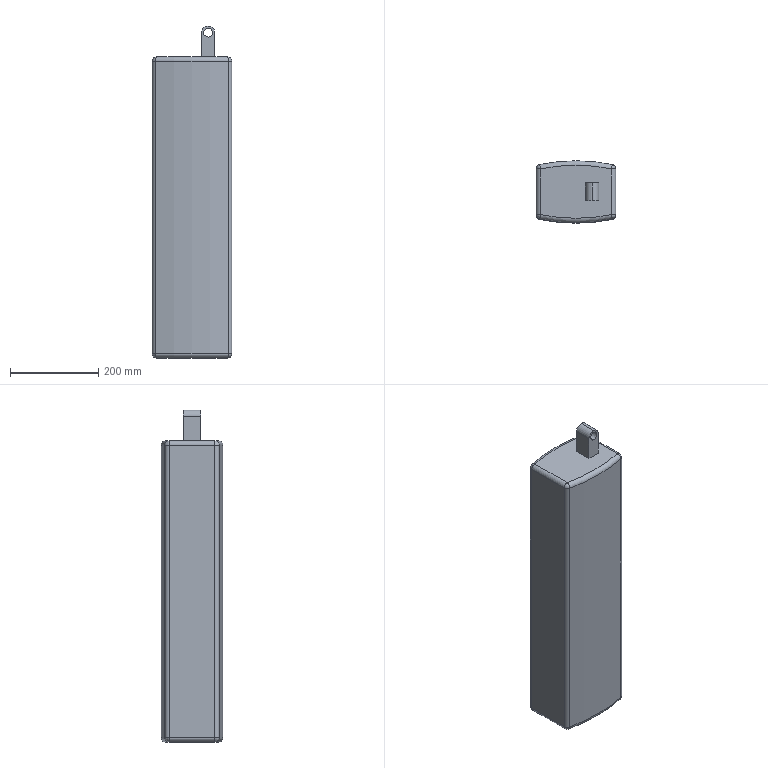Part | STEP file | LASER HEAD D120I | 1 solid | 34 faces | box 180 x 140 x 751 mm | volume 16335319 mm3 | cylinder 14 | plane 8 | sphere 8 | torus 4 | commonest cylinder face diameters 20 x10 30 x2 800 x2
STEP:
#1=CARTESIAN_POINT('',(89.923,-16.765,746.));
#2=VERTEX_POINT('',#1);
#3=CARTESIAN_POINT('',(89.923,-16.765,726.));
#4=VERTEX_POINT('',#3);
#5=CARTESIAN_POINT('',(89.923,-16.765,736.));
#6=DIRECTION('',(0.,-1.,0.));
#7=DIRECTION('',(1.,0.,0.));
#8=AXIS2_PLACEMENT_3D('',#5,#6,#7);
#9=CIRCLE('',#8,10.);
#10=EDGE_CURVE('',#2,#4,#9,.T.);
#11=ORIENTED_EDGE('',*,*,#10,.F.);
#12=CARTESIAN_POINT('',(89.923,-56.765,746.));
#13=VERTEX_POINT('',#12);
#14=CARTESIAN_POINT('',(89.923,13.235,746.));
#15=DIRECTION('',(0.,-1.,0.));
#16=VECTOR('',#15,1000.);
#17=LINE('',#14,#16);
#18=EDGE_CURVE('',#2,#13,#17,.T.);
#19=ORIENTED_EDGE('',*,*,#18,.T.);
#20=CARTESIAN_POINT('',(89.923,-56.765,726.));
#21=VERTEX_POINT('',#20);
#22=CARTESIAN_POINT('',(89.923,-56.765,736.));
#23=DIRECTION('',(0.,-1.,0.));
#24=DIRECTION('',(0.,0.,-1.));
#25=AXIS2_PLACEMENT_3D('',#22,#23,#24);
#26=CIRCLE('',#25,10.);
#27=EDGE_CURVE('',#13,#21,#26,.T.);
#28=ORIENTED_EDGE('',*,*,#27,.T.);
#29=CARTESIAN_POINT('',(89.923,13.235,726.));
#30=DIRECTION('',(0.,-1.,0.));
#31=VECTOR('',#30,1000.);
#32=LINE('',#29,#31);
#33=EDGE_CURVE('',#4,#21,#32,.T.);
#34=ORIENTED_EDGE('',*,*,#33,.F.);
#35=EDGE_LOOP('',(#11,#19,#28,#34));
#36=FACE_OUTER_BOUND('',#35,.T.);
#37=CARTESIAN_POINT('',(89.923,13.235,736.));
#38=DIRECTION('',(0.,-1.,0.));
#39=DIRECTION('',(0.,0.,-1.));
#40=AXIS2_PLACEMENT_3D('',#37,#38,#39);
#41=CYLINDRICAL_SURFACE('',#40,10.);
#42=ADVANCED_FACE('',(#36),#41,.F.);
#43=CARTESIAN_POINT('',(133.454,-88.42,681.));
#44=VERTEX_POINT('',#43);
#45=CARTESIAN_POINT('',(133.454,14.889,681.));
#46=VERTEX_POINT('',#45);
#47=CARTESIAN_POINT('',(133.454,-88.42,681.));
#48=DIRECTION('',(0.,1.,0.));
#49=VECTOR('',#48,1000.);
#50=LINE('',#47,#49);
#51=EDGE_CURVE('',#44,#46,#50,.T.);
#52=ORIENTED_EDGE('',*,*,#51,.T.);
#53=CARTESIAN_POINT('',(-26.546,14.994,681.));
#54=VERTEX_POINT('',#53);
#55=CARTESIAN_POINT('',(53.205,-366.765,681.));
#56=DIRECTION('',(0.,0.,1.));
#57=DIRECTION('',(-1.,0.,0.));
#58=AXIS2_PLACEMENT_3D('',#55,#56,#57);
#59=CIRCLE('',#58,390.);
#60=EDGE_CURVE('',#46,#54,#59,.T.);
#61=ORIENTED_EDGE('',*,*,#60,.T.);
#62=CARTESIAN_POINT('',(-26.546,-88.524,681.));
#63=VERTEX_POINT('',#62);
#64=CARTESIAN_POINT('',(-26.546,-88.42,681.));
#65=DIRECTION('',(0.,-1.,0.));
#66=VECTOR('',#65,1000.);
#67=LINE('',#64,#66);
#68=EDGE_CURVE('',#54,#63,#67,.T.);
#69=ORIENTED_EDGE('',*,*,#68,.T.);
#70=CARTESIAN_POINT('',(53.205,293.235,681.));
#71=DIRECTION('',(0.,0.,1.));
#72=DIRECTION('',(-1.,0.,0.));
#73=AXIS2_PLACEMENT_3D('',#70,#71,#72);
#74=CIRCLE('',#73,390.);
#75=EDGE_CURVE('',#63,#44,#74,.T.);
#76=ORIENTED_EDGE('',*,*,#75,.T.);
#77=EDGE_LOOP('',(#52,#61,#69,#76));
#78=FACE_OUTER_BOUND('',#77,.T.);
#79=CARTESIAN_POINT('',(74.923,-16.765,681.));
#80=VERTEX_POINT('',#79);
#81=CARTESIAN_POINT('',(74.923,-56.765,681.));
#82=VERTEX_POINT('',#81);
#83=CARTESIAN_POINT('',(74.923,-16.765,681.));
#84=DIRECTION('',(0.,-1.,0.));
#85=VECTOR('',#84,1000.);
#86=LINE('',#83,#85);
#87=EDGE_CURVE('',#80,#82,#86,.T.);
#88=ORIENTED_EDGE('',*,*,#87,.F.);
#89=CARTESIAN_POINT('',(104.923,-16.765,681.));
#90=VERTEX_POINT('',#89);
#91=CARTESIAN_POINT('',(74.923,-16.765,681.));
#92=DIRECTION('',(-1.,0.,0.));
#93=VECTOR('',#92,1000.);
#94=LINE('',#91,#93);
#95=EDGE_CURVE('',#90,#80,#94,.T.);
#96=ORIENTED_EDGE('',*,*,#95,.F.);
#97=CARTESIAN_POINT('',(104.923,-56.765,681.));
#98=VERTEX_POINT('',#97);
#99=CARTESIAN_POINT('',(104.923,-16.765,681.));
#100=DIRECTION('',(0.,1.,0.));
#101=VECTOR('',#100,1000.);
#102=LINE('',#99,#101);
#103=EDGE_CURVE('',#98,#90,#102,.T.);
#104=ORIENTED_EDGE('',*,*,#103,.F.);
#105=CARTESIAN_POINT('',(74.923,-56.765,681.));
#106=DIRECTION('',(1.,0.,0.));
#107=VECTOR('',#106,1000.);
#108=LINE('',#105,#107);
#109=EDGE_CURVE('',#82,#98,#108,.T.);
#110=ORIENTED_EDGE('',*,*,#109,.F.);
#111=EDGE_LOOP('',(#88,#96,#104,#110));
#112=FACE_BOUND('',#111,.T.);
#113=CARTESIAN_POINT('',(133.454,-88.42,681.));
#114=DIRECTION('',(0.,0.,-1.));
#115=DIRECTION('',(-1.,0.,0.));
#116=AXIS2_PLACEMENT_3D('',#113,#114,#115);
#117=PLANE('',#116);
#118=ADVANCED_FACE('',(#78,#112),#117,.F.);
#119=CARTESIAN_POINT('',(143.454,-88.42,671.));
#120=VERTEX_POINT('',#119);
#121=CARTESIAN_POINT('',(143.454,-88.42,10.));
#122=VERTEX_POINT('',#121);
#123=CARTESIAN_POINT('',(143.454,-88.42,681.));
#124=DIRECTION('',(0.,0.,-1.));
#125=VECTOR('',#124,1000.);
#126=LINE('',#123,#125);
#127=EDGE_CURVE('',#120,#122,#126,.T.);
#128=ORIENTED_EDGE('',*,*,#127,.F.);
#129=CARTESIAN_POINT('',(135.512,-98.206,671.));
#130=VERTEX_POINT('',#129);
#131=CARTESIAN_POINT('',(133.454,-88.42,671.));
#132=DIRECTION('',(0.,0.,-1.));
#133=DIRECTION('',(-1.,0.,0.));
#134=AXIS2_PLACEMENT_3D('',#131,#132,#133);
#135=CIRCLE('',#134,10.);
#136=EDGE_CURVE('',#120,#130,#135,.T.);
#137=ORIENTED_EDGE('',*,*,#136,.T.);
#138=CARTESIAN_POINT('',(135.512,-98.206,10.));
#139=VERTEX_POINT('',#138);
#140=CARTESIAN_POINT('',(135.512,-98.206,681.));
#141=DIRECTION('',(0.,0.,-1.));
#142=VECTOR('',#141,1000.);
#143=LINE('',#140,#142);
#144=EDGE_CURVE('',#130,#139,#143,.T.);
#145=ORIENTED_EDGE('',*,*,#144,.T.);
#146=CARTESIAN_POINT('',(133.454,-88.42,10.));
#147=DIRECTION('',(0.,0.,1.));
#148=DIRECTION('',(-1.,0.,0.));
#149=AXIS2_PLACEMENT_3D('',#146,#147,#148);
#150=CIRCLE('',#149,10.);
#151=EDGE_CURVE('',#139,#122,#150,.T.);
#152=ORIENTED_EDGE('',*,*,#151,.T.);
#153=EDGE_LOOP('',(#128,#137,#145,#152));
#154=FACE_OUTER_BOUND('',#153,.T.);
#155=CARTESIAN_POINT('',(133.454,-88.42,681.));
#156=DIRECTION('',(0.,0.,-1.));
#157=DIRECTION('',(-1.,0.,0.));
#158=AXIS2_PLACEMENT_3D('',#155,#156,#157);
#159=CYLINDRICAL_SURFACE('',#158,10.);
#160=ADVANCED_FACE('',(#154),#159,.T.);
#161=CARTESIAN_POINT('',(143.454,14.889,671.));
#162=VERTEX_POINT('',#161);
#163=CARTESIAN_POINT('',(143.454,14.889,10.));
#164=VERTEX_POINT('',#163);
#165=CARTESIAN_POINT('',(143.454,14.889,681.));
#166=DIRECTION('',(0.,0.,-1.));
#167=VECTOR('',#166,1000.);
#168=LINE('',#165,#167);
#169=EDGE_CURVE('',#162,#164,#168,.T.);
#170=ORIENTED_EDGE('',*,*,#169,.F.);
#171=CARTESIAN_POINT('',(143.454,14.889,671.));
#172=DIRECTION('',(0.,-1.,0.));
#173=VECTOR('',#172,1000.);
#174=LINE('',#171,#173);
#175=EDGE_CURVE('',#162,#120,#174,.T.);
#176=ORIENTED_EDGE('',*,*,#175,.T.);
#177=ORIENTED_EDGE('',*,*,#127,.T.);
#178=CARTESIAN_POINT('',(143.454,14.889,10.));
#179=DIRECTION('',(0.,1.,0.));
#180=VECTOR('',#179,1000.);
#181=LINE('',#178,#180);
#182=EDGE_CURVE('',#122,#164,#181,.T.);
#183=ORIENTED_EDGE('',*,*,#182,.T.);
#184=EDGE_LOOP('',(#170,#176,#177,#183));
#185=FACE_OUTER_BOUND('',#184,.T.);
#186=CARTESIAN_POINT('',(143.454,14.889,681.));
#187=DIRECTION('',(-1.,0.,0.));
#188=DIRECTION('',(0.,0.,1.));
#189=AXIS2_PLACEMENT_3D('',#186,#187,#188);
#190=PLANE('',#189);
#191=ADVANCED_FACE('',(#185),#190,.F.);
#192=CARTESIAN_POINT('',(135.512,24.675,671.));
#193=VERTEX_POINT('',#192);
#194=CARTESIAN_POINT('',(135.512,24.675,10.));
#195=VERTEX_POINT('',#194);
#196=CARTESIAN_POINT('',(135.512,24.675,681.));
#197=DIRECTION('',(0.,0.,-1.));
#198=VECTOR('',#197,1000.);
#199=LINE('',#196,#198);
#200=EDGE_CURVE('',#193,#195,#199,.T.);
#201=ORIENTED_EDGE('',*,*,#200,.F.);
#202=CARTESIAN_POINT('',(133.454,14.889,671.));
#203=DIRECTION('',(0.,0.,-1.));
#204=DIRECTION('',(-1.,0.,0.));
#205=AXIS2_PLACEMENT_3D('',#202,#203,#204);
#206=CIRCLE('',#205,10.);
#207=EDGE_CURVE('',#193,#162,#206,.T.);
#208=ORIENTED_EDGE('',*,*,#207,.T.);
#209=ORIENTED_EDGE('',*,*,#169,.T.);
#210=CARTESIAN_POINT('',(133.454,14.889,10.));
#211=DIRECTION('',(0.,0.,1.));
#212=DIRECTION('',(-1.,0.,0.));
#213=AXIS2_PLACEMENT_3D('',#210,#211,#212);
#214=CIRCLE('',#213,10.);
#215=EDGE_CURVE('',#164,#195,#214,.T.);
#216=ORIENTED_EDGE('',*,*,#215,.T.);
#217=EDGE_LOOP('',(#201,#208,#209,#216));
#218=FACE_OUTER_BOUND('',#217,.T.);
#219=CARTESIAN_POINT('',(133.454,14.889,681.));
#220=DIRECTION('',(0.,0.,-1.));
#221=DIRECTION('',(-1.,0.,0.));
#222=AXIS2_PLACEMENT_3D('',#219,#220,#221);
#223=CYLINDRICAL_SURFACE('',#222,10.);
#224=ADVANCED_FACE('',(#218),#223,.T.);
#225=CARTESIAN_POINT('',(-28.591,24.782,671.));
#226=VERTEX_POINT('',#225);
#227=CARTESIAN_POINT('',(-28.591,24.782,10.));
#228=VERTEX_POINT('',#227);
#229=CARTESIAN_POINT('',(-28.591,24.782,681.));
#230=DIRECTION('',(0.,0.,-1.));
#231=VECTOR('',#230,1000.);
#232=LINE('',#229,#231);
#233=EDGE_CURVE('',#226,#228,#232,.T.);
#234=ORIENTED_EDGE('',*,*,#233,.F.);
#235=CARTESIAN_POINT('',(53.205,-366.765,671.));
#236=DIRECTION('',(0.,0.,-1.));
#237=DIRECTION('',(-1.,0.,0.));
#238=AXIS2_PLACEMENT_3D('',#235,#236,#237);
#239=CIRCLE('',#238,400.);
#240=EDGE_CURVE('',#226,#193,#239,.T.);
#241=ORIENTED_EDGE('',*,*,#240,.T.);
#242=ORIENTED_EDGE('',*,*,#200,.T.);
#243=CARTESIAN_POINT('',(53.205,-366.765,10.));
#244=DIRECTION('',(0.,0.,1.));
#245=DIRECTION('',(-1.,0.,0.));
#246=AXIS2_PLACEMENT_3D('',#243,#244,#245);
#247=CIRCLE('',#246,400.);
#248=EDGE_CURVE('',#195,#228,#247,.T.);
#249=ORIENTED_EDGE('',*,*,#248,.T.);
#250=EDGE_LOOP('',(#234,#241,#242,#249));
#251=FACE_OUTER_BOUND('',#250,.T.);
#252=CARTESIAN_POINT('',(53.205,-366.765,681.));
#253=DIRECTION('',(0.,0.,-1.));
#254=DIRECTION('',(-1.,0.,0.));
#255=AXIS2_PLACEMENT_3D('',#252,#253,#254);
#256=CYLINDRICAL_SURFACE('',#255,400.);
#257=ADVANCED_FACE('',(#251),#256,.T.);
#258=CARTESIAN_POINT('',(-36.546,14.994,671.));
#259=VERTEX_POINT('',#258);
#260=CARTESIAN_POINT('',(-36.546,14.994,10.));
#261=VERTEX_POINT('',#260);
#262=CARTESIAN_POINT('',(-36.546,14.994,681.));
#263=DIRECTION('',(0.,0.,-1.));
#264=VECTOR('',#263,1000.);
#265=LINE('',#262,#264);
#266=EDGE_CURVE('',#259,#261,#265,.T.);
#267=ORIENTED_EDGE('',*,*,#266,.F.);
#268=CARTESIAN_POINT('',(-26.546,14.994,671.));
#269=DIRECTION('',(0.,0.,-1.));
#270=DIRECTION('',(-1.,0.,0.));
#271=AXIS2_PLACEMENT_3D('',#268,#269,#270);
#272=CIRCLE('',#271,10.);
#273=EDGE_CURVE('',#259,#226,#272,.T.);
#274=ORIENTED_EDGE('',*,*,#273,.T.);
#275=ORIENTED_EDGE('',*,*,#233,.T.);
#276=CARTESIAN_POINT('',(-26.546,14.994,10.));
#277=DIRECTION('',(0.,0.,1.));
#278=DIRECTION('',(-1.,0.,0.));
#279=AXIS2_PLACEMENT_3D('',#276,#277,#278);
#280=CIRCLE('',#279,10.);
#281=EDGE_CURVE('',#228,#261,#280,.T.);
#282=ORIENTED_EDGE('',*,*,#281,.T.);
#283=EDGE_LOOP('',(#267,#274,#275,#282));
#284=FACE_OUTER_BOUND('',#283,.T.);
#285=CARTESIAN_POINT('',(-26.546,14.994,681.));
#286=DIRECTION('',(0.,0.,-1.));
#287=DIRECTION('',(-1.,0.,0.));
#288=AXIS2_PLACEMENT_3D('',#285,#286,#287);
#289=CYLINDRICAL_SURFACE('',#288,10.);
#290=ADVANCED_FACE('',(#284),#289,.T.);
#291=CARTESIAN_POINT('',(-36.546,-88.524,671.));
#292=VERTEX_POINT('',#291);
#293=CARTESIAN_POINT('',(-36.546,-88.524,10.));
#294=VERTEX_POINT('',#293);
#295=CARTESIAN_POINT('',(-36.546,-88.524,681.));
#296=DIRECTION('',(0.,0.,-1.));
#297=VECTOR('',#296,1000.);
#298=LINE('',#295,#297);
#299=EDGE_CURVE('',#292,#294,#298,.T.);
#300=ORIENTED_EDGE('',*,*,#299,.F.);
#301=CARTESIAN_POINT('',(-36.546,14.994,671.));
#302=DIRECTION('',(0.,1.,0.));
#303=VECTOR('',#302,1000.);
#304=LINE('',#301,#303);
#305=EDGE_CURVE('',#292,#259,#304,.T.);
#306=ORIENTED_EDGE('',*,*,#305,.T.);
#307=ORIENTED_EDGE('',*,*,#266,.T.);
#308=CARTESIAN_POINT('',(-36.546,-88.524,10.));
#309=DIRECTION('',(0.,-1.,0.));
#310=VECTOR('',#309,1000.);
#311=LINE('',#308,#310);
#312=EDGE_CURVE('',#261,#294,#311,.T.);
#313=ORIENTED_EDGE('',*,*,#312,.T.);
#314=EDGE_LOOP('',(#300,#306,#307,#313));
#315=FACE_OUTER_BOUND('',#314,.T.);
#316=CARTESIAN_POINT('',(-36.546,14.994,681.));
#317=DIRECTION('',(1.,0.,0.));
#318=DIRECTION('',(0.,0.,-1.));
#319=AXIS2_PLACEMENT_3D('',#316,#317,#318);
#320=PLANE('',#319);
#321=ADVANCED_FACE('',(#315),#320,.F.);
#322=CARTESIAN_POINT('',(-28.591,-98.313,671.));
#323=VERTEX_POINT('',#322);
#324=CARTESIAN_POINT('',(-28.591,-98.313,10.));
#325=VERTEX_POINT('',#324);
#326=CARTESIAN_POINT('',(-28.591,-98.313,681.));
#327=DIRECTION('',(0.,0.,-1.));
#328=VECTOR('',#327,1000.);
#329=LINE('',#326,#328);
#330=EDGE_CURVE('',#323,#325,#329,.T.);
#331=ORIENTED_EDGE('',*,*,#330,.F.);
#332=CARTESIAN_POINT('',(-26.546,-88.524,671.));
#333=DIRECTION('',(0.,0.,-1.));
#334=DIRECTION('',(-1.,0.,0.));
#335=AXIS2_PLACEMENT_3D('',#332,#333,#334);
#336=CIRCLE('',#335,10.);
#337=EDGE_CURVE('',#323,#292,#336,.T.);
#338=ORIENTED_EDGE('',*,*,#337,.T.);
#339=ORIENTED_EDGE('',*,*,#299,.T.);
#340=CARTESIAN_POINT('',(-26.546,-88.524,10.));
#341=DIRECTION('',(0.,0.,1.));
#342=DIRECTION('',(-1.,0.,0.));
#343=AXIS2_PLACEMENT_3D('',#340,#341,#342);
#344=CIRCLE('',#343,10.);
#345=EDGE_CURVE('',#294,#325,#344,.T.);
#346=ORIENTED_EDGE('',*,*,#345,.T.);
#347=EDGE_LOOP('',(#331,#338,#339,#346));
#348=FACE_OUTER_BOUND('',#347,.T.);
#349=CARTESIAN_POINT('',(-26.546,-88.524,681.));
#350=DIRECTION('',(0.,0.,-1.));
#351=DIRECTION('',(-1.,0.,0.));
#352=AXIS2_PLACEMENT_3D('',#349,#350,#351);
#353=CYLINDRICAL_SURFACE('',#352,10.);
#354=ADVANCED_FACE('',(#348),#353,.T.);
#355=ORIENTED_EDGE('',*,*,#144,.F.);
#356=CARTESIAN_POINT('',(53.205,293.235,671.));
#357=DIRECTION('',(0.,0.,-1.));
#358=DIRECTION('',(-1.,0.,0.));
#359=AXIS2_PLACEMENT_3D('',#356,#357,#358);
#360=CIRCLE('',#359,400.);
#361=EDGE_CURVE('',#130,#323,#360,.T.);
#362=ORIENTED_EDGE('',*,*,#361,.T.);
#363=ORIENTED_EDGE('',*,*,#330,.T.);
#364=CARTESIAN_POINT('',(53.205,293.235,10.));
#365=DIRECTION('',(0.,0.,1.));
#366=DIRECTION('',(-1.,0.,0.));
#367=AXIS2_PLACEMENT_3D('',#364,#365,#366);
#368=CIRCLE('',#367,400.);
#369=EDGE_CURVE('',#325,#139,#368,.T.);
#370=ORIENTED_EDGE('',*,*,#369,.T.);
#371=EDGE_LOOP('',(#355,#362,#363,#370));
#372=FACE_OUTER_BOUND('',#371,.T.);
#373=CARTESIAN_POINT('',(53.205,293.235,681.));
#374=DIRECTION('',(0.,0.,-1.));
#375=DIRECTION('',(-1.,0.,0.));
#376=AXIS2_PLACEMENT_3D('',#373,#374,#375);
#377=CYLINDRICAL_SURFACE('',#376,400.);
#378=ADVANCED_FACE('',(#372),#377,.T.);
#379=CARTESIAN_POINT('',(-26.546,-88.524,0.));
#380=VERTEX_POINT('',#379);
#381=CARTESIAN_POINT('',(-26.546,14.994,0.));
#382=VERTEX_POINT('',#381);
#383=CARTESIAN_POINT('',(-26.546,14.994,0.));
#384=DIRECTION('',(0.,1.,0.));
#385=VECTOR('',#384,1000.);
#386=LINE('',#383,#385);
#387=EDGE_CURVE('',#380,#382,#386,.T.);
#388=ORIENTED_EDGE('',*,*,#387,.T.);
#389=CARTESIAN_POINT('',(133.454,14.889,0.));
#390=VERTEX_POINT('',#389);
#391=CARTESIAN_POINT('',(53.205,-366.765,0.));
#392=DIRECTION('',(0.,0.,-1.));
#393=DIRECTION('',(-1.,0.,0.));
#394=AXIS2_PLACEMENT_3D('',#391,#392,#393);
#395=CIRCLE('',#394,390.);
#396=EDGE_CURVE('',#382,#390,#395,.T.);
#397=ORIENTED_EDGE('',*,*,#396,.T.);
#398=CARTESIAN_POINT('',(133.454,-88.42,0.));
#399=VERTEX_POINT('',#398);
#400=CARTESIAN_POINT('',(133.454,-88.42,0.));
#401=DIRECTION('',(0.,-1.,0.));
#402=VECTOR('',#401,1000.);
#403=LINE('',#400,#402);
#404=EDGE_CURVE('',#390,#399,#403,.T.);
#405=ORIENTED_EDGE('',*,*,#404,.T.);
#406=CARTESIAN_POINT('',(53.205,293.235,0.));
#407=DIRECTION('',(0.,0.,-1.));
#408=DIRECTION('',(-1.,0.,0.));
#409=AXIS2_PLACEMENT_3D('',#406,#407,#408);
#410=CIRCLE('',#409,390.);
#411=EDGE_CURVE('',#399,#380,#410,.T.);
#412=ORIENTED_EDGE('',*,*,#411,.T.);
#413=EDGE_LOOP('',(#388,#397,#405,#412));
#414=FACE_OUTER_BOUND('',#413,.T.);
#415=CARTESIAN_POINT('',(133.454,-88.42,0.));
#416=DIRECTION('',(0.,0.,-1.));
#417=DIRECTION('',(-1.,0.,0.));
#418=AXIS2_PLACEMENT_3D('',#415,#416,#417);
#419=PLANE('',#418);
#420=ADVANCED_FACE('',(#414),#419,.T.);
#421=CARTESIAN_POINT('',(133.454,-88.42,671.));
#422=DIRECTION('',(-0.9786,-0.2058,0.));
#423=DIRECTION('',(0.2058,-0.9786,0.));
#424=AXIS2_PLACEMENT_3D('',#421,#422,#423);
#425=CIRCLE('',#424,10.);
#426=EDGE_CURVE('',#130,#44,#425,.T.);
#427=ORIENTED_EDGE('',*,*,#426,.F.);
#428=ORIENTED_EDGE('',*,*,#136,.F.);
#429=CARTESIAN_POINT('',(133.454,-88.42,671.));
#430=DIRECTION('',(0.,1.,0.));
#431=DIRECTION('',(0.,0.,1.));
#432=AXIS2_PLACEMENT_3D('',#429,#430,#431);
#433=CIRCLE('',#432,10.);
#434=EDGE_CURVE('',#44,#120,#433,.T.);
#435=ORIENTED_EDGE('',*,*,#434,.F.);
#436=EDGE_LOOP('',(#427,#428,#435));
#437=FACE_OUTER_BOUND('',#436,.T.);
#438=CARTESIAN_POINT('',(133.454,-88.42,671.));
#439=DIRECTION('',(0.,1.,0.));
#440=DIRECTION('',(1.,0.,0.));
#441=AXIS2_PLACEMENT_3D('',#438,#439,#440);
#442=SPHERICAL_SURFACE('',#441,10.);
#443=ADVANCED_FACE('',(#437),#442,.T.);
#444=ORIENTED_EDGE('',*,*,#434,.T.);
#445=ORIENTED_EDGE('',*,*,#175,.F.);
#446=CARTESIAN_POINT('',(133.454,14.889,671.));
#447=DIRECTION('',(0.,1.,0.));
#448=DIRECTION('',(0.,0.,1.));
#449=AXIS2_PLACEMENT_3D('',#446,#447,#448);
#450=CIRCLE('',#449,10.);
#451=EDGE_CURVE('',#46,#162,#450,.T.);
#452=ORIENTED_EDGE('',*,*,#451,.F.);
#453=ORIENTED_EDGE('',*,*,#51,.F.);
#454=EDGE_LOOP('',(#444,#445,#452,#453));
#455=FACE_OUTER_BOUND('',#454,.T.);
#456=CARTESIAN_POINT('',(133.454,-88.42,671.));
#457=DIRECTION('',(0.,1.,0.));
#458=DIRECTION('',(0.,0.,1.));
#459=AXIS2_PLACEMENT_3D('',#456,#457,#458);
#460=CYLINDRICAL_SURFACE('',#459,10.);
#461=ADVANCED_FACE('',(#455),#460,.T.);
#462=ORIENTED_EDGE('',*,*,#426,.T.);
#463=ORIENTED_EDGE('',*,*,#75,.F.);
#464=CARTESIAN_POINT('',(-26.546,-88.524,671.));
#465=DIRECTION('',(-0.9789,0.2045,0.));
#466=DIRECTION('',(-0.2045,-0.9789,0.));
#467=AXIS2_PLACEMENT_3D('',#464,#465,#466);
#468=CIRCLE('',#467,10.);
#469=EDGE_CURVE('',#323,#63,#468,.T.);
#470=ORIENTED_EDGE('',*,*,#469,.F.);
#471=ORIENTED_EDGE('',*,*,#361,.F.);
#472=EDGE_LOOP('',(#462,#463,#470,#471));
#473=FACE_OUTER_BOUND('',#472,.T.);
#474=CARTESIAN_POINT('',(53.205,293.235,671.));
#475=DIRECTION('',(0.,0.,-1.));
#476=DIRECTION('',(-1.,0.,0.));
#477=AXIS2_PLACEMENT_3D('',#474,#475,#476);
#478=TOROIDAL_SURFACE('',#477,390.,10.);
#479=ADVANCED_FACE('',(#473),#478,.T.);
#480=ORIENTED_EDGE('',*,*,#451,.T.);
#481=ORIENTED_EDGE('',*,*,#207,.F.);
#482=CARTESIAN_POINT('',(133.454,14.889,671.));
#483=DIRECTION('',(-0.9786,0.2058,0.));
#484=DIRECTION('',(-0.2058,-0.9786,0.));
#485=AXIS2_PLACEMENT_3D('',#482,#483,#484);
#486=CIRCLE('',#485,10.);
#487=EDGE_CURVE('',#46,#193,#486,.T.);
#488=ORIENTED_EDGE('',*,*,#487,.F.);
#489=EDGE_LOOP('',(#480,#481,#488));
#490=FACE_OUTER_BOUND('',#489,.T.);
#491=CARTESIAN_POINT('',(133.454,14.889,671.));
#492=DIRECTION('',(0.,1.,0.));
#493=DIRECTION('',(1.,0.,0.));
#494=AXIS2_PLACEMENT_3D('',#491,#492,#493);
#495=SPHERICAL_SURFACE('',#494,10.);
#496=ADVANCED_FACE('',(#490),#495,.T.);
#497=ORIENTED_EDGE('',*,*,#337,.F.);
#498=ORIENTED_EDGE('',*,*,#469,.T.);
#499=CARTESIAN_POINT('',(-26.546,-88.524,671.));
#500=DIRECTION('',(0.,1.,0.));
#501=DIRECTION('',(0.,0.,1.));
#502=AXIS2_PLACEMENT_3D('',#499,#500,#501);
#503=CIRCLE('',#502,10.);
#504=EDGE_CURVE('',#292,#63,#503,.T.);
#505=ORIENTED_EDGE('',*,*,#504,.F.);
#506=EDGE_LOOP('',(#497,#498,#505));
#507=FACE_OUTER_BOUND('',#506,.T.);
#508=CARTESIAN_POINT('',(-26.546,-88.524,671.));
#509=DIRECTION('',(0.,1.,0.));
#510=DIRECTION('',(1.,0.,0.));
#511=AXIS2_PLACEMENT_3D('',#508,#509,#510);
#512=SPHERICAL_SURFACE('',#511,10.);
#513=ADVANCED_FACE('',(#507),#512,.T.);
#514=ORIENTED_EDGE('',*,*,#487,.T.);
#515=ORIENTED_EDGE('',*,*,#240,.F.);
#516=CARTESIAN_POINT('',(-26.546,14.994,671.));
#517=DIRECTION('',(-0.9789,-0.2045,0.));
#518=DIRECTION('',(0.2045,-0.9789,0.));
#519=AXIS2_PLACEMENT_3D('',#516,#517,#518);
#520=CIRCLE('',#519,10.);
#521=EDGE_CURVE('',#54,#226,#520,.T.);
#522=ORIENTED_EDGE('',*,*,#521,.F.);
#523=ORIENTED_EDGE('',*,*,#60,.F.);
#524=EDGE_LOOP('',(#514,#515,#522,#523));
#525=FACE_OUTER_BOUND('',#524,.T.);
#526=CARTESIAN_POINT('',(53.205,-366.765,671.));
#527=DIRECTION('',(0.,0.,-1.));
#528=DIRECTION('',(-1.,0.,0.));
#529=AXIS2_PLACEMENT_3D('',#526,#527,#528);
#530=TOROIDAL_SURFACE('',#529,390.,10.);
#531=ADVANCED_FACE('',(#525),#530,.T.);
#532=ORIENTED_EDGE('',*,*,#504,.T.);
#533=ORIENTED_EDGE('',*,*,#68,.F.);
#534=CARTESIAN_POINT('',(-26.546,14.994,671.));
#535=DIRECTION('',(0.,1.,0.));
#536=DIRECTION('',(0.,0.,1.));
#537=AXIS2_PLACEMENT_3D('',#534,#535,#536);
#538=CIRCLE('',#537,10.);
#539=EDGE_CURVE('',#259,#54,#538,.T.);
#540=ORIENTED_EDGE('',*,*,#539,.F.);
#541=ORIENTED_EDGE('',*,*,#305,.F.);
#542=EDGE_LOOP('',(#532,#533,#540,#541));
#543=FACE_OUTER_BOUND('',#542,.T.);
#544=CARTESIAN_POINT('',(-26.546,-88.42,671.));
#545=DIRECTION('',(0.,-1.,0.));
#546=DIRECTION('',(0.,0.,-1.));
#547=AXIS2_PLACEMENT_3D('',#544,#545,#546);
#548=CYLINDRICAL_SURFACE('',#547,10.);
#549=ADVANCED_FACE('',(#543),#548,.T.);
#550=ORIENTED_EDGE('',*,*,#521,.T.);
#551=ORIENTED_EDGE('',*,*,#273,.F.);
#552=ORIENTED_EDGE('',*,*,#539,.T.);
#553=EDGE_LOOP('',(#550,#551,#552));
#554=FACE_OUTER_BOUND('',#553,.T.);
#555=CARTESIAN_POINT('',(-26.546,14.994,671.));
#556=DIRECTION('',(0.,1.,0.));
#557=DIRECTION('',(1.,0.,0.));
#558=AXIS2_PLACEMENT_3D('',#555,#556,#557);
#559=SPHERICAL_SURFACE('',#558,10.);
#560=ADVANCED_FACE('',(#554),#559,.T.);
#561=CARTESIAN_POINT('',(133.454,-88.42,10.));
#562=DIRECTION('',(-0.9786,-0.2058,0.));
#563=DIRECTION('',(0.2058,-0.9786,0.));
#564=AXIS2_PLACEMENT_3D('',#561,#562,#563);
#565=CIRCLE('',#564,10.);
#566=EDGE_CURVE('',#399,#139,#565,.T.);
#567=ORIENTED_EDGE('',*,*,#566,.F.);
#568=CARTESIAN_POINT('',(133.454,-88.42,10.));
#569=DIRECTION('',(0.,1.,0.));
#570=DIRECTION('',(0.,0.,1.));
#571=AXIS2_PLACEMENT_3D('',#568,#569,#570);
#572=CIRCLE('',#571,10.);
#573=EDGE_CURVE('',#122,#399,#572,.T.);
#574=ORIENTED_EDGE('',*,*,#573,.F.);
#575=ORIENTED_EDGE('',*,*,#151,.F.);
#576=EDGE_LOOP('',(#567,#574,#575));
#577=FACE_OUTER_BOUND('',#576,.T.);
#578=CARTESIAN_POINT('',(133.454,-88.42,10.));
#579=DIRECTION('',(0.,1.,0.));
#580=DIRECTION('',(1.,0.,0.));
#581=AXIS2_PLACEMENT_3D('',#578,#579,#580);
#582=SPHERICAL_SURFACE('',#581,10.);
#583=ADVANCED_FACE('',(#577),#582,.T.);
#584=ORIENTED_EDGE('',*,*,#573,.T.);
#585=ORIENTED_EDGE('',*,*,#404,.F.);
#586=CARTESIAN_POINT('',(133.454,14.889,10.));
#587=DIRECTION('',(0.,1.,0.));
#588=DIRECTION('',(0.,0.,1.));
#589=AXIS2_PLACEMENT_3D('',#586,#587,#588);
#590=CIRCLE('',#589,10.);
#591=EDGE_CURVE('',#164,#390,#590,.T.);
#592=ORIENTED_EDGE('',*,*,#591,.F.);
#593=ORIENTED_EDGE('',*,*,#182,.F.);
#594=EDGE_LOOP('',(#584,#585,#592,#593));
#595=FACE_OUTER_BOUND('',#594,.T.);
#596=CARTESIAN_POINT('',(133.454,14.889,10.));
#597=DIRECTION('',(0.,-1.,0.));
#598=DIRECTION('',(0.,0.,-1.));
#599=AXIS2_PLACEMENT_3D('',#596,#597,#598);
#600=CYLINDRICAL_SURFACE('',#599,10.);
#601=ADVANCED_FACE('',(#595),#600,.T.);
#602=ORIENTED_EDGE('',*,*,#566,.T.);
#603=ORIENTED_EDGE('',*,*,#369,.F.);
#604=CARTESIAN_POINT('',(-26.546,-88.524,10.));
#605=DIRECTION('',(-0.9789,0.2045,0.));
#606=DIRECTION('',(-0.2045,-0.9789,0.));
#607=AXIS2_PLACEMENT_3D('',#604,#605,#606);
#608=CIRCLE('',#607,10.);
#609=EDGE_CURVE('',#380,#325,#608,.T.);
#610=ORIENTED_EDGE('',*,*,#609,.F.);
#611=ORIENTED_EDGE('',*,*,#411,.F.);
#612=EDGE_LOOP('',(#602,#603,#610,#611));
#613=FACE_OUTER_BOUND('',#612,.T.);
#614=CARTESIAN_POINT('',(53.205,293.235,10.));
#615=DIRECTION('',(0.,0.,-1.));
#616=DIRECTION('',(-1.,0.,0.));
#617=AXIS2_PLACEMENT_3D('',#614,#615,#616);
#618=TOROIDAL_SURFACE('',#617,390.,10.);
#619=ADVANCED_FACE('',(#613),#618,.T.);
#620=ORIENTED_EDGE('',*,*,#215,.F.);
#621=ORIENTED_EDGE('',*,*,#591,.T.);
#622=CARTESIAN_POINT('',(133.454,14.889,10.));
#623=DIRECTION('',(-0.9786,0.2058,0.));
#624=DIRECTION('',(-0.2058,-0.9786,0.));
#625=AXIS2_PLACEMENT_3D('',#622,#623,#624);
#626=CIRCLE('',#625,10.);
#627=EDGE_CURVE('',#195,#390,#626,.T.);
#628=ORIENTED_EDGE('',*,*,#627,.F.);
#629=EDGE_LOOP('',(#620,#621,#628));
#630=FACE_OUTER_BOUND('',#629,.T.);
#631=CARTESIAN_POINT('',(133.454,14.889,10.));
#632=DIRECTION('',(0.,1.,0.));
#633=DIRECTION('',(1.,0.,0.));
#634=AXIS2_PLACEMENT_3D('',#631,#632,#633);
#635=SPHERICAL_SURFACE('',#634,10.);
#636=ADVANCED_FACE('',(#630),#635,.T.);
#637=ORIENTED_EDGE('',*,*,#609,.T.);
#638=ORIENTED_EDGE('',*,*,#345,.F.);
#639=CARTESIAN_POINT('',(-26.546,-88.524,10.));
#640=DIRECTION('',(0.,1.,0.));
#641=DIRECTION('',(0.,0.,1.));
#642=AXIS2_PLACEMENT_3D('',#639,#640,#641);
#643=CIRCLE('',#642,10.);
#644=EDGE_CURVE('',#380,#294,#643,.T.);
#645=ORIENTED_EDGE('',*,*,#644,.F.);
#646=EDGE_LOOP('',(#637,#638,#645));
#647=FACE_OUTER_BOUND('',#646,.T.);
#648=CARTESIAN_POINT('',(-26.546,-88.524,10.));
#649=DIRECTION('',(0.,1.,0.));
#650=DIRECTION('',(1.,0.,0.));
#651=AXIS2_PLACEMENT_3D('',#648,#649,#650);
#652=SPHERICAL_SURFACE('',#651,10.);
#653=ADVANCED_FACE('',(#647),#652,.T.);
#654=ORIENTED_EDGE('',*,*,#627,.T.);
#655=ORIENTED_EDGE('',*,*,#396,.F.);
#656=CARTESIAN_POINT('',(-26.546,14.994,10.));
#657=DIRECTION('',(-0.9789,-0.2045,0.));
#658=DIRECTION('',(0.2045,-0.9789,0.));
#659=AXIS2_PLACEMENT_3D('',#656,#657,#658);
#660=CIRCLE('',#659,10.);
#661=EDGE_CURVE('',#228,#382,#660,.T.);
#662=ORIENTED_EDGE('',*,*,#661,.F.);
#663=ORIENTED_EDGE('',*,*,#248,.F.);
#664=EDGE_LOOP('',(#654,#655,#662,#663));
#665=FACE_OUTER_BOUND('',#664,.T.);
#666=CARTESIAN_POINT('',(53.205,-366.765,10.));
#667=DIRECTION('',(0.,0.,-1.));
#668=DIRECTION('',(-1.,0.,0.));
#669=AXIS2_PLACEMENT_3D('',#666,#667,#668);
#670=TOROIDAL_SURFACE('',#669,390.,10.);
#671=ADVANCED_FACE('',(#665),#670,.T.);
#672=ORIENTED_EDGE('',*,*,#644,.T.);
#673=ORIENTED_EDGE('',*,*,#312,.F.);
#674=CARTESIAN_POINT('',(-26.546,14.994,10.));
#675=DIRECTION('',(0.,1.,0.));
#676=DIRECTION('',(-1.,0.,0.));
#677=AXIS2_PLACEMENT_3D('',#674,#675,#676);
#678=CIRCLE('',#677,10.);
#679=EDGE_CURVE('',#382,#261,#678,.T.);
#680=ORIENTED_EDGE('',*,*,#679,.F.);
#681=ORIENTED_EDGE('',*,*,#387,.F.);
#682=EDGE_LOOP('',(#672,#673,#680,#681));
#683=FACE_OUTER_BOUND('',#682,.T.);
#684=CARTESIAN_POINT('',(-26.546,14.994,10.));
#685=DIRECTION('',(0.,1.,0.));
#686=DIRECTION('',(0.,0.,1.));
#687=AXIS2_PLACEMENT_3D('',#684,#685,#686);
#688=CYLINDRICAL_SURFACE('',#687,10.);
#689=ADVANCED_FACE('',(#683),#688,.T.);
#690=ORIENTED_EDGE('',*,*,#281,.F.);
#691=ORIENTED_EDGE('',*,*,#661,.T.);
#692=ORIENTED_EDGE('',*,*,#679,.T.);
#693=EDGE_LOOP('',(#690,#691,#692));
#694=FACE_OUTER_BOUND('',#693,.T.);
#695=CARTESIAN_POINT('',(-26.546,14.994,10.));
#696=DIRECTION('',(0.,1.,0.));
#697=DIRECTION('',(1.,0.,0.));
#698=AXIS2_PLACEMENT_3D('',#695,#696,#697);
#699=SPHERICAL_SURFACE('',#698,10.);
#700=ADVANCED_FACE('',(#694),#699,.T.);
#701=CARTESIAN_POINT('',(74.923,-56.765,736.));
#702=VERTEX_POINT('',#701);
#703=CARTESIAN_POINT('',(74.923,-56.765,751.));
#704=DIRECTION('',(0.,0.,-1.));
#705=VECTOR('',#704,1000.);
#706=LINE('',#703,#705);
#707=EDGE_CURVE('',#702,#82,#706,.T.);
#708=ORIENTED_EDGE('',*,*,#707,.F.);
#709=CARTESIAN_POINT('',(74.923,-16.765,736.));
#710=VERTEX_POINT('',#709);
#711=CARTESIAN_POINT('',(74.923,-16.765,736.));
#712=DIRECTION('',(0.,1.,0.));
#713=VECTOR('',#712,1000.);
#714=LINE('',#711,#713);
#715=EDGE_CURVE('',#702,#710,#714,.T.);
#716=ORIENTED_EDGE('',*,*,#715,.T.);
#717=CARTESIAN_POINT('',(74.923,-16.765,751.));
#718=DIRECTION('',(0.,0.,-1.));
#719=VECTOR('',#718,1000.);
#720=LINE('',#717,#719);
#721=EDGE_CURVE('',#710,#80,#720,.T.);
#722=ORIENTED_EDGE('',*,*,#721,.T.);
#723=ORIENTED_EDGE('',*,*,#87,.T.);
#724=EDGE_LOOP('',(#708,#716,#722,#723));
#725=FACE_OUTER_BOUND('',#724,.T.);
#726=CARTESIAN_POINT('',(74.923,-16.765,751.));
#727=DIRECTION('',(1.,0.,0.));
#728=DIRECTION('',(0.,1.,0.));
#729=AXIS2_PLACEMENT_3D('',#726,#727,#728);
#730=PLANE('',#729);
#731=ADVANCED_FACE('',(#725),#730,.F.);
#732=CARTESIAN_POINT('',(89.923,-56.765,736.));
#733=DIRECTION('',(0.,-1.,0.));
#734=DIRECTION('',(0.,0.,-1.));
#735=AXIS2_PLACEMENT_3D('',#732,#733,#734);
#736=CIRCLE('',#735,10.);
#737=EDGE_CURVE('',#21,#13,#736,.T.);
#738=ORIENTED_EDGE('',*,*,#737,.F.);
#739=ORIENTED_EDGE('',*,*,#27,.F.);
#740=EDGE_LOOP('',(#738,#739));
#741=FACE_BOUND('',#740,.T.);
#742=CARTESIAN_POINT('',(104.923,-56.765,736.));
#743=VERTEX_POINT('',#742);
#744=CARTESIAN_POINT('',(104.923,-56.765,751.));
#745=DIRECTION('',(0.,0.,-1.));
#746=VECTOR('',#745,1000.);
#747=LINE('',#744,#746);
#748=EDGE_CURVE('',#743,#98,#747,.T.);
#749=ORIENTED_EDGE('',*,*,#748,.F.);
#750=CARTESIAN_POINT('',(89.923,-56.765,751.));
#751=VERTEX_POINT('',#750);
#752=CARTESIAN_POINT('',(89.923,-56.765,736.));
#753=DIRECTION('',(0.,-1.,0.));
#754=DIRECTION('',(0.,0.,1.));
#755=AXIS2_PLACEMENT_3D('',#752,#753,#754);
#756=CIRCLE('',#755,15.);
#757=EDGE_CURVE('',#743,#751,#756,.T.);
#758=ORIENTED_EDGE('',*,*,#757,.T.);
#759=CARTESIAN_POINT('',(89.923,-56.765,736.));
#760=DIRECTION('',(0.,-1.,0.));
#761=DIRECTION('',(0.,0.,1.));
#762=AXIS2_PLACEMENT_3D('',#759,#760,#761);
#763=CIRCLE('',#762,15.);
#764=EDGE_CURVE('',#751,#702,#763,.T.);
#765=ORIENTED_EDGE('',*,*,#764,.T.);
#766=ORIENTED_EDGE('',*,*,#707,.T.);
#767=ORIENTED_EDGE('',*,*,#109,.T.);
#768=EDGE_LOOP('',(#749,#758,#765,#766,#767));
#769=FACE_OUTER_BOUND('',#768,.T.);
#770=CARTESIAN_POINT('',(74.923,-56.765,751.));
#771=DIRECTION('',(0.,1.,0.));
#772=DIRECTION('',(0.,0.,1.));
#773=AXIS2_PLACEMENT_3D('',#770,#771,#772);
#774=PLANE('',#773);
#775=ADVANCED_FACE('',(#741,#769),#774,.F.);
#776=CARTESIAN_POINT('',(104.923,-16.765,736.));
#777=VERTEX_POINT('',#776);
#778=CARTESIAN_POINT('',(104.923,-16.765,751.));
#779=DIRECTION('',(0.,0.,-1.));
#780=VECTOR('',#779,1000.);
#781=LINE('',#778,#780);
#782=EDGE_CURVE('',#777,#90,#781,.T.);
#783=ORIENTED_EDGE('',*,*,#782,.F.);
#784=CARTESIAN_POINT('',(104.923,-56.765,736.));
#785=DIRECTION('',(0.,-1.,0.));
#786=VECTOR('',#785,1000.);
#787=LINE('',#784,#786);
#788=EDGE_CURVE('',#777,#743,#787,.T.);
#789=ORIENTED_EDGE('',*,*,#788,.T.);
#790=ORIENTED_EDGE('',*,*,#748,.T.);
#791=ORIENTED_EDGE('',*,*,#103,.T.);
#792=EDGE_LOOP('',(#783,#789,#790,#791));
#793=FACE_OUTER_BOUND('',#792,.T.);
#794=CARTESIAN_POINT('',(104.923,-16.765,751.));
#795=DIRECTION('',(-1.,0.,0.));
#796=DIRECTION('',(0.,0.,1.));
#797=AXIS2_PLACEMENT_3D('',#794,#795,#796);
#798=PLANE('',#797);
#799=ADVANCED_FACE('',(#793),#798,.F.);
#800=CARTESIAN_POINT('',(89.923,-16.765,736.));
#801=DIRECTION('',(0.,-1.,0.));
#802=DIRECTION('',(1.,0.,0.));
#803=AXIS2_PLACEMENT_3D('',#800,#801,#802);
#804=CIRCLE('',#803,10.);
#805=EDGE_CURVE('',#4,#2,#804,.T.);
#806=ORIENTED_EDGE('',*,*,#805,.T.);
#807=ORIENTED_EDGE('',*,*,#10,.T.);
#808=EDGE_LOOP('',(#806,#807));
#809=FACE_BOUND('',#808,.T.);
#810=CARTESIAN_POINT('',(89.923,-16.765,751.));
#811=VERTEX_POINT('',#810);
#812=CARTESIAN_POINT('',(89.923,-16.765,736.));
#813=DIRECTION('',(0.,1.,0.));
#814=DIRECTION('',(1.,0.,0.));
#815=AXIS2_PLACEMENT_3D('',#812,#813,#814);
#816=CIRCLE('',#815,15.);
#817=EDGE_CURVE('',#710,#811,#816,.T.);
#818=ORIENTED_EDGE('',*,*,#817,.T.);
#819=CARTESIAN_POINT('',(89.923,-16.765,736.));
#820=DIRECTION('',(0.,1.,0.));
#821=DIRECTION('',(1.,0.,0.));
#822=AXIS2_PLACEMENT_3D('',#819,#820,#821);
#823=CIRCLE('',#822,15.);
#824=EDGE_CURVE('',#811,#777,#823,.T.);
#825=ORIENTED_EDGE('',*,*,#824,.T.);
#826=ORIENTED_EDGE('',*,*,#782,.T.);
#827=ORIENTED_EDGE('',*,*,#95,.T.);
#828=ORIENTED_EDGE('',*,*,#721,.F.);
#829=EDGE_LOOP('',(#818,#825,#826,#827,#828));
#830=FACE_OUTER_BOUND('',#829,.T.);
#831=CARTESIAN_POINT('',(74.923,-16.765,751.));
#832=DIRECTION('',(0.,-1.,0.));
#833=DIRECTION('',(1.,0.,0.));
#834=AXIS2_PLACEMENT_3D('',#831,#832,#833);
#835=PLANE('',#834);
#836=ADVANCED_FACE('',(#809,#830),#835,.F.);
#837=ORIENTED_EDGE('',*,*,#715,.F.);
#838=ORIENTED_EDGE('',*,*,#764,.F.);
#839=CARTESIAN_POINT('',(89.923,-56.765,751.));
#840=DIRECTION('',(0.,-1.,0.));
#841=VECTOR('',#840,1000.);
#842=LINE('',#839,#841);
#843=EDGE_CURVE('',#811,#751,#842,.T.);
#844=ORIENTED_EDGE('',*,*,#843,.F.);
#845=ORIENTED_EDGE('',*,*,#817,.F.);
#846=EDGE_LOOP('',(#837,#838,#844,#845));
#847=FACE_OUTER_BOUND('',#846,.T.);
#848=CARTESIAN_POINT('',(89.923,-56.765,736.));
#849=DIRECTION('',(0.,1.,0.));
#850=DIRECTION('',(-1.,0.,0.));
#851=AXIS2_PLACEMENT_3D('',#848,#849,#850);
#852=CYLINDRICAL_SURFACE('',#851,15.);
#853=ADVANCED_FACE('',(#847),#852,.T.);
#854=ORIENTED_EDGE('',*,*,#757,.F.);
#855=ORIENTED_EDGE('',*,*,#788,.F.);
#856=ORIENTED_EDGE('',*,*,#824,.F.);
#857=ORIENTED_EDGE('',*,*,#843,.T.);
#858=EDGE_LOOP('',(#854,#855,#856,#857));
#859=FACE_OUTER_BOUND('',#858,.T.);
#860=CARTESIAN_POINT('',(89.923,-56.765,736.));
#861=DIRECTION('',(0.,-1.,0.));
#862=DIRECTION('',(0.,0.,-1.));
#863=AXIS2_PLACEMENT_3D('',#860,#861,#862);
#864=CYLINDRICAL_SURFACE('',#863,15.);
#865=ADVANCED_FACE('',(#859),#864,.T.);
#866=ORIENTED_EDGE('',*,*,#18,.F.);
#867=ORIENTED_EDGE('',*,*,#805,.F.);
#868=ORIENTED_EDGE('',*,*,#33,.T.);
#869=ORIENTED_EDGE('',*,*,#737,.T.);
#870=EDGE_LOOP('',(#866,#867,#868,#869));
#871=FACE_OUTER_BOUND('',#870,.T.);
#872=CARTESIAN_POINT('',(89.923,13.235,736.));
#873=DIRECTION('',(0.,-1.,0.));
#874=DIRECTION('',(0.,0.,-1.));
#875=AXIS2_PLACEMENT_3D('',#872,#873,#874);
#876=CYLINDRICAL_SURFACE('',#875,10.);
#877=ADVANCED_FACE('',(#871),#876,.F.);
#878=CLOSED_SHELL('',(#42,#118,#160,#191,#224,#257,#290,#321,#354,#378,#420,#443,#461,#479,#496,#513,#531,#549,#560,#583,#601,#619,#636,#653,#671,#689,#700,#731,#775,#799,#836,#853,#865,#877));
#879=MANIFOLD_SOLID_BREP('',#878);
#880=CARTESIAN_POINT('',(0.,0.,0.));
#881=DIRECTION('',(0.,0.,1.));
#882=DIRECTION('',(1.,0.,0.));
#883=AXIS2_PLACEMENT_3D('',#880,#881,#882);
#884=(LENGTH_UNIT()NAMED_UNIT(*)SI_UNIT(.MILLI.,.METRE.));
#885=UNCERTAINTY_MEASURE_WITH_UNIT(LENGTH_MEASURE(0.00001),#884,'','');
#886=(NAMED_UNIT(*)PLANE_ANGLE_UNIT()SI_UNIT($,.RADIAN.));
#887=(NAMED_UNIT(*)SI_UNIT($,.STERADIAN.)SOLID_ANGLE_UNIT());
#888=(GEOMETRIC_REPRESENTATION_CONTEXT(3)GLOBAL_UNCERTAINTY_ASSIGNED_CONTEXT((#885))GLOBAL_UNIT_ASSIGNED_CONTEXT((#884,#886,#887))REPRESENTATION_CONTEXT('',''));
#889=ADVANCED_BREP_SHAPE_REPRESENTATION('',(#879,#883),#888);